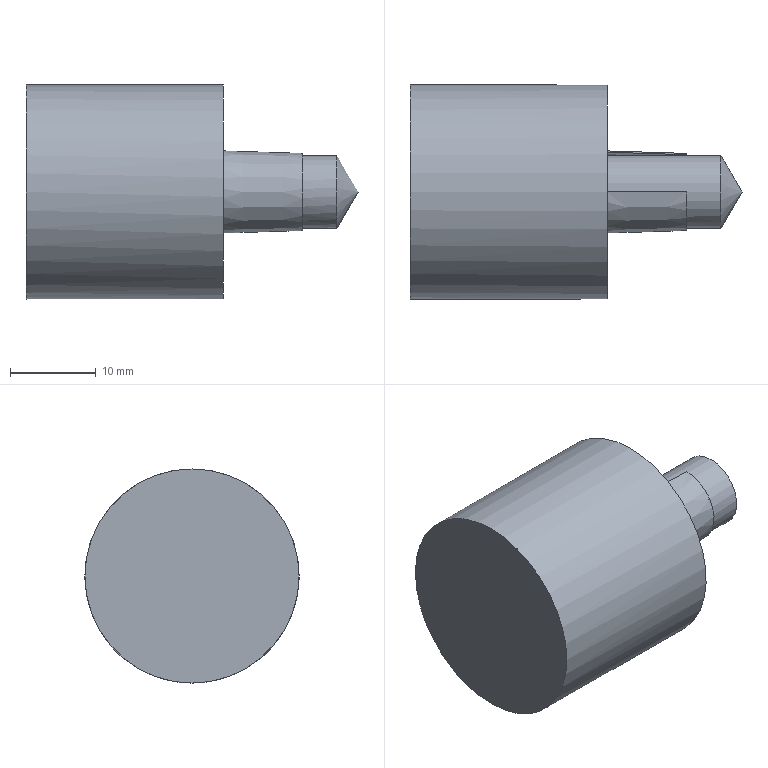Part | NX | features solid 2 | 1 solid | 68 faces | box 38.754 x 25 x 25 mm | volume 12122 mm3 | spline 28 | plane 27 | cylinder 10 | cone 3 | commonest cylinder face diameters 8.7 x5 8.5 x4 25 x1